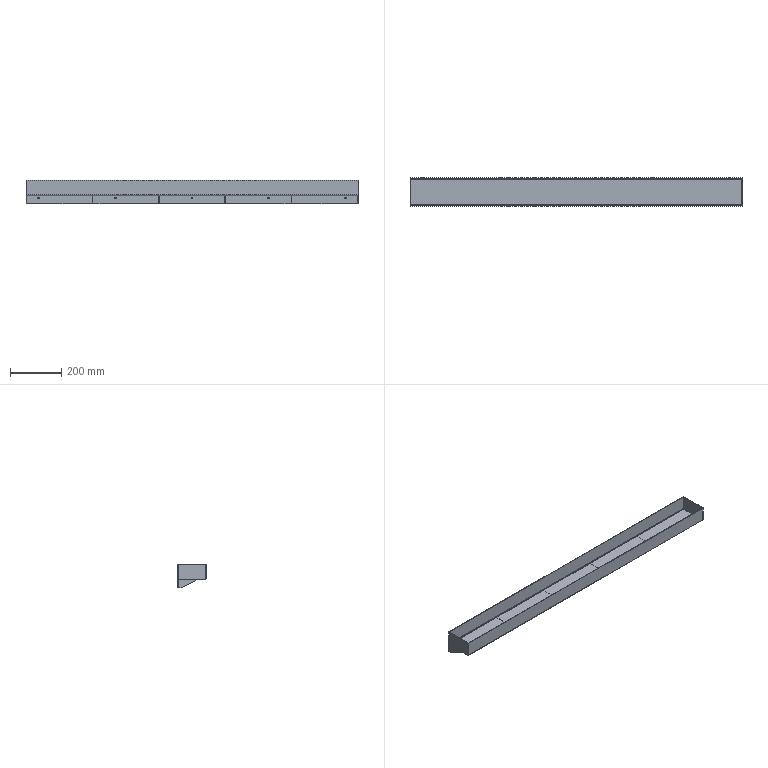Part | STEP file | Sheet box 1300 | 1 solid | 57 faces | box 1300 x 110 x 92 mm | volume 708554 mm3 | plane 39 | cylinder 18 | commonest cylinder face diameters 6.5 x10 10 x6 6 x2